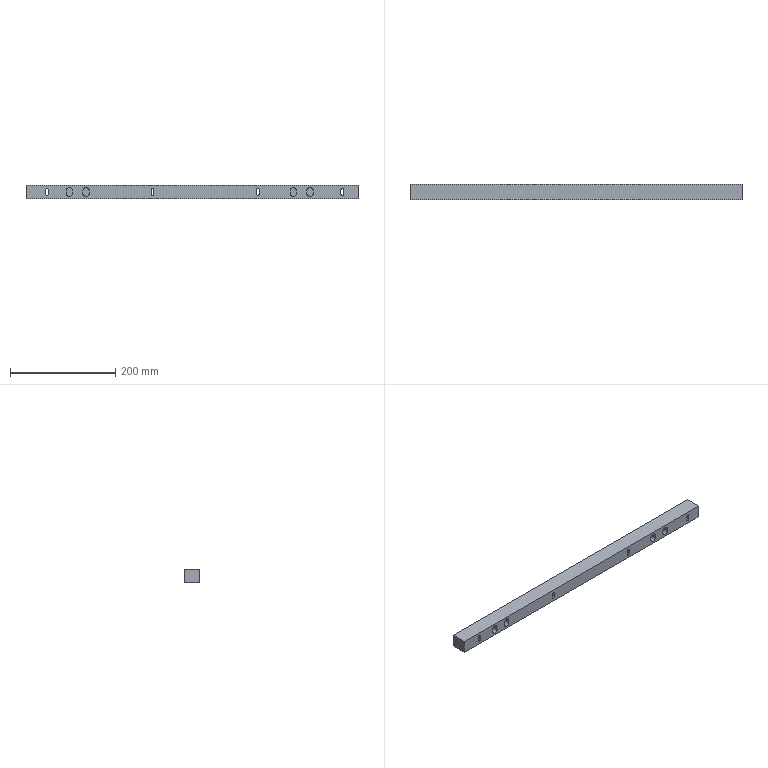Part | STEP file | 0243_218_Bar | 1 solid | 66 faces | box 630 x 30 x 25 mm | volume 456558 mm3 | cylinder 32 | plane 26 | cone 8 | commonest cylinder face diameters 5.5 x12 12 x12 5 x8